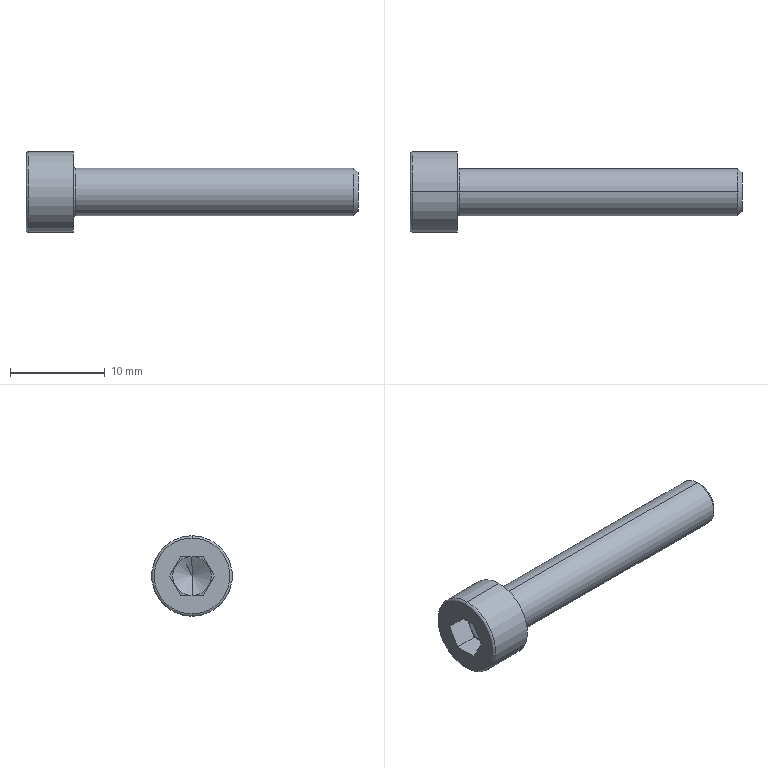Part | STEP file | PN_0056_socket head screw-M5x35 | 1 solid | 27 faces | box 35 x 8.5 x 8.5 mm | volume 829.835 mm3 | plane 15 | cone 4 | torus 4 | cylinder 4 | commonest cylinder face diameters 5 x2 8.5 x2